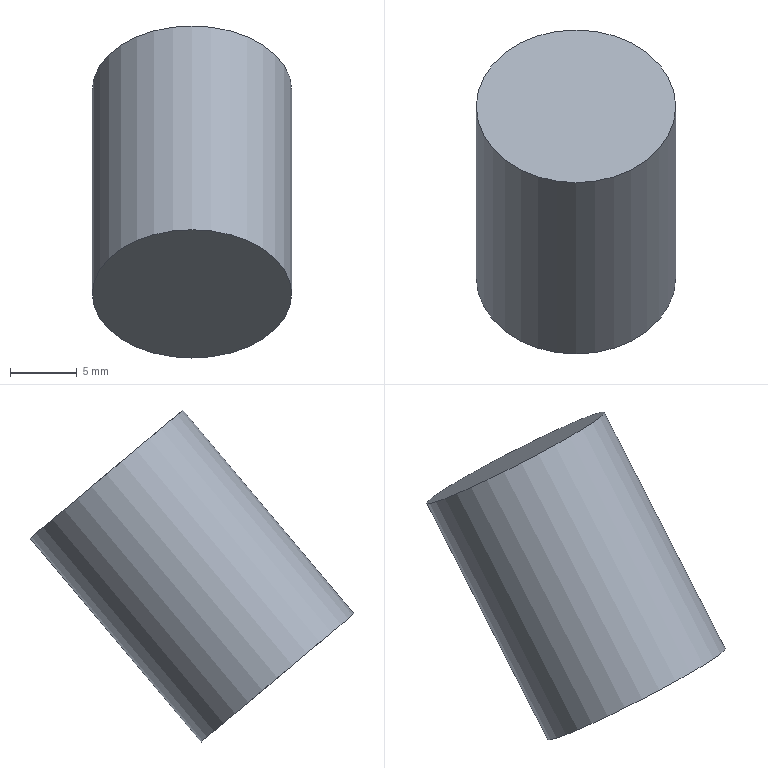Part | NX | features solid 2 | 1 solid | 3 faces | box 15 x 24.346 x 24.963 mm | volume 3534 mm3 | plane 2 | cylinder 1 | commonest cylinder face diameters 15 x1
STEP:
#1=CARTESIAN_POINT('',(297.5,427.179,-43.19));
#2=VERTEX_POINT('',#1);
#3=CARTESIAN_POINT('',(305.,427.179,-43.19));
#4=DIRECTION('',(0.,0.6428,0.766));
#5=DIRECTION('',(-1.,0.,0.));
#6=AXIS2_PLACEMENT_3D('',#3,#4,#5);
#7=CIRCLE('',#6,7.5);
#8=EDGE_CURVE('',#2,#2,#7,.T.);
#9=ORIENTED_EDGE('',*,*,#8,.T.);
#10=EDGE_LOOP('',(#9));
#11=FACE_BOUND('',#10,.T.);
#12=CARTESIAN_POINT('',(305.,427.179,-43.19));
#13=DIRECTION('',(0.,0.6428,0.766));
#14=DIRECTION('',(0.,-0.766,0.6428));
#15=AXIS2_PLACEMENT_3D('',#12,#13,#14);
#16=PLANE('',#15);
#17=ADVANCED_FACE('',(#11),#16,.T.);
#18=CARTESIAN_POINT('',(312.5,414.323,-58.511));
#19=VERTEX_POINT('',#18);
#20=CARTESIAN_POINT('',(305.,414.323,-58.511));
#21=DIRECTION('',(0.,-0.6428,-0.766));
#22=DIRECTION('',(1.,0.,0.));
#23=AXIS2_PLACEMENT_3D('',#20,#21,#22);
#24=CIRCLE('',#23,7.5);
#25=EDGE_CURVE('',#19,#19,#24,.F.);
#26=ORIENTED_EDGE('',*,*,#25,.T.);
#27=EDGE_LOOP('',(#26));
#28=FACE_BOUND('',#27,.T.);
#29=ORIENTED_EDGE('',*,*,#8,.F.);
#30=EDGE_LOOP('',(#29));
#31=FACE_BOUND('',#30,.T.);
#32=CARTESIAN_POINT('',(305.,423.322,-47.786));
#33=DIRECTION('',(0.,-0.6428,-0.766));
#34=DIRECTION('',(0.,0.766,-0.6428));
#35=AXIS2_PLACEMENT_3D('',#32,#33,#34);
#36=CYLINDRICAL_SURFACE('',#35,7.5);
#37=ADVANCED_FACE('',(#28,#31),#36,.T.);
#38=ORIENTED_EDGE('',*,*,#25,.F.);
#39=EDGE_LOOP('',(#38));
#40=FACE_BOUND('',#39,.T.);
#41=CARTESIAN_POINT('',(305.,414.323,-58.511));
#42=DIRECTION('',(0.,0.6428,0.766));
#43=DIRECTION('',(0.,-0.766,0.6428));
#44=AXIS2_PLACEMENT_3D('',#41,#42,#43);
#45=PLANE('',#44);
#46=ADVANCED_FACE('',(#40),#45,.F.);
#47=CLOSED_SHELL('',(#17,#37,#46));
#48=MANIFOLD_SOLID_BREP('',#47);
#49=(LENGTH_UNIT()NAMED_UNIT(*)SI_UNIT(.MILLI.,.METRE.));
#50=UNCERTAINTY_MEASURE_WITH_UNIT(LENGTH_MEASURE(0.00001),#49,'','');
#51=(NAMED_UNIT(*)PLANE_ANGLE_UNIT()SI_UNIT($,.RADIAN.));
#52=(NAMED_UNIT(*)SI_UNIT($,.STERADIAN.)SOLID_ANGLE_UNIT());
#53=(GEOMETRIC_REPRESENTATION_CONTEXT(3)GLOBAL_UNCERTAINTY_ASSIGNED_CONTEXT((#50))GLOBAL_UNIT_ASSIGNED_CONTEXT((#49,#51,#52))REPRESENTATION_CONTEXT('',''));
#54=ADVANCED_BREP_SHAPE_REPRESENTATION('',(#48),#53);